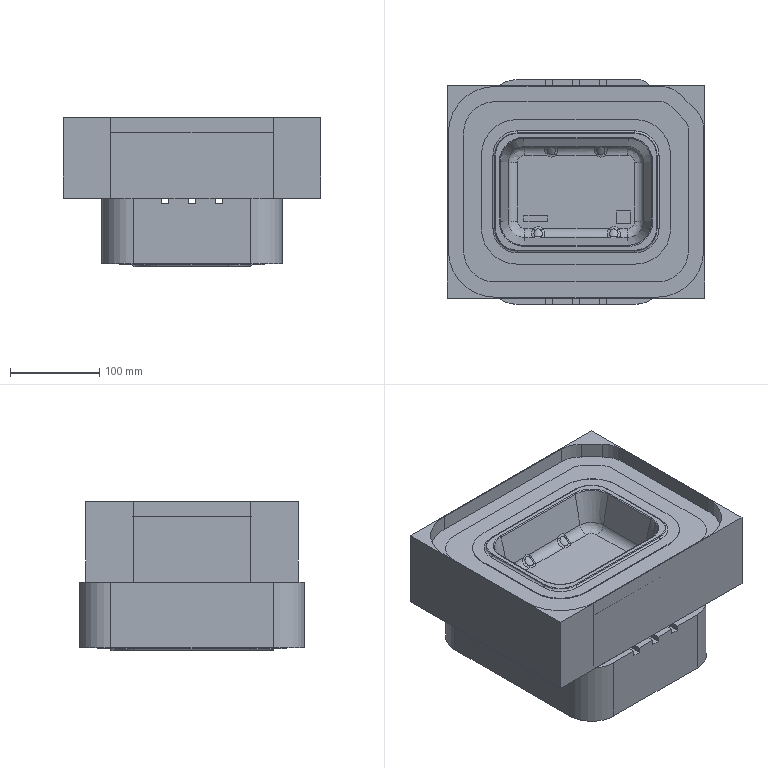NC program | NX | posted with a generic post | part box 287.436 x 251.436 x 167.016 mm
Lines 1 to 1276 of 118587:
N10 G17 G21 G94 G90
(01 , TOOL : D16R0.8)
N12 T00 M6
N14 G53
N16 G17 G0 G90 X27.566 Y-109.658 S7000 M3 M8
N18 G43 Z240.5 H0
N20 Z91.5
N22 G94 G1 X0. Z90.055 F4500.
N24 X-90.718
N26 G2 X-134.583 Y-65.793 R43.865
N28 G1 Y65.793
N30 G2 X-90.718 Y109.658 R43.865
N32 G1 X94.505
N34 G2 X111.38 Y102.668 R23.865
N36 G1 X127.593 Y86.455
N38 G2 X134.583 Y69.58 R23.865
N40 G1 Y-65.793
N42 G2 X90.718 Y-109.658 R43.865
N44 G1 X0.
N46 Y-99.578
N48 X-90.718
N50 G2 X-124.503 Y-65.793 R33.785
N52 G1 Y65.793
N54 G2 X-90.718 Y99.578 R33.785
N56 G1 X94.505
N58 G2 X104.252 Y95.541 R13.785
N60 G1 X120.466 Y79.327
N62 G2 X124.503 Y69.58 R13.785
N64 G1 Y-65.793
N66 G2 X90.718 Y-99.578 R33.785
N68 G1 X0.
N70 Y-89.498
N72 X-90.718
N74 G2 X-114.423 Y-65.793 R23.705
N76 G1 Y65.793
N78 G2 X-90.718 Y89.498 R23.705
N80 G1 X94.505
N82 G2 X97.125 Y88.413 R3.705
N84 G1 X113.338 Y72.2
N86 G2 X114.423 Y69.58 R3.705
N88 G1 Y-65.793
N90 G2 X90.718 Y-89.498 R23.705
N92 G1 X0.
N94 Y-79.418
N96 X-90.718
N98 G2 X-104.343 Y-65.793 R13.625
N100 G1 Y65.793
N102 G2 X-90.718 Y79.418 R13.625
N104 G1 X91.864
N106 X104.343 Y66.939
N108 Y-65.793
N110 G2 X90.718 Y-79.418 R13.625
N112 G1 X0.
N114 Y-69.338
N116 X-90.718
N118 G2 X-94.263 Y-65.793 R3.545
N120 G1 Y65.793
N122 G2 X-90.718 Y69.338 R3.545
N124 G1 X87.689
N126 X94.263 Y62.764
N128 Y-65.793
N130 G2 X90.718 Y-69.338 R3.545
N132 G1 X0.
N134 Y-59.258
N136 X-84.183
N138 Y59.258
N140 X83.514
N142 X84.183 Y58.589
N144 Y-59.258
N146 X0.
N148 Y-49.178
N150 X-74.103
N152 Y49.178
N154 X74.103
N156 Y-49.178
N158 X0.
N160 Y-39.098
N162 X-64.023
N164 Y39.098
N166 X64.023
N168 Y-39.098
N170 X0.
N172 Y-29.018
N174 X-53.943
N176 Y29.018
N178 X53.943
N180 Y-29.018
N182 X0.
N184 Y-18.938
N186 X-43.863
N188 Y18.938
N190 X43.863
N192 Y-18.938
N194 X0.
N196 Y-8.858
N198 X-33.783
N200 Y8.858
N202 X33.783
N204 Y-8.858
N206 X0.
N208 Y-1.658
N210 X-26.583
N212 Y1.658
N214 X26.583
N216 Y-1.658
N218 X0.
N220 G3 X-3.2 Y-4.858 R3.2
N222 G1 Z91.055
N224 G0 Z93.5
N226 X27.566 Y-109.593
N228 Z91.055
N230 G1 X0. Z89.611
N232 X-90.718
N234 G2 X-134.518 Y-65.793 R43.8
N236 G1 Y65.793
N238 G2 X-90.718 Y109.593 R43.8
N240 G1 X94.505
N242 G2 X111.334 Y102.622 R23.8
N244 G1 X127.547 Y86.409
N246 G2 X134.518 Y69.58 R23.8
N248 G1 Y-65.793
N250 G2 X90.718 Y-109.593 R43.8
N252 G1 X0.
N254 Y-99.513
N256 X-90.718
N258 G2 X-124.438 Y-65.793 R33.72
N260 G1 Y65.793
N262 G2 X-90.718 Y99.513 R33.72
N264 G1 X94.505
N266 G2 X104.206 Y95.495 R13.72
N268 G1 X120.42 Y79.281
N270 G2 X124.438 Y69.58 R13.72
N272 G1 Y-65.793
N274 G2 X90.718 Y-99.513 R33.72
N276 G1 X0.
N278 Y-89.433
N280 X-90.718
N282 G2 X-114.358 Y-65.793 R23.64
N284 G1 Y65.793
N286 G2 X-90.718 Y89.433 R23.64
N288 G1 X94.505
N290 G2 X97.079 Y88.367 R3.64
N292 G1 X113.292 Y72.154
N294 G2 X114.358 Y69.58 R3.64
N296 G1 Y-65.793
N298 G2 X90.718 Y-89.433 R23.64
N300 G1 X0.
N302 Y-79.353
N304 X-90.718
N306 G2 X-104.278 Y-65.793 R13.56
N308 G1 Y65.793
N310 G2 X-90.718 Y79.353 R13.56
N312 G1 X91.837
N314 X104.278 Y66.912
N316 Y-65.793
N318 G2 X90.718 Y-79.353 R13.56
N320 G1 X0.
N322 Y-69.273
N324 X-90.718
N326 G2 X-94.198 Y-65.793 R3.48
N328 G1 Y65.793
N330 G2 X-90.718 Y69.273 R3.48
N332 G1 X87.662
N334 X94.198 Y62.737
N336 Y-65.793
N338 G2 X90.718 Y-69.273 R3.48
N340 G1 X0.
N342 Y-59.193
N344 X-84.118
N346 Y59.193
N348 X83.487
N350 X84.118 Y58.562
N352 Y-59.193
N354 X0.
N356 Y-49.113
N358 X-74.038
N360 Y49.113
N362 X74.038
N364 Y-49.113
N366 X0.
N368 Y-39.033
N370 X-63.958
N372 Y39.033
N374 X63.958
N376 Y-39.033
N378 X0.
N380 Y-28.953
N382 X-53.878
N384 Y28.953
N386 X53.878
N388 Y-28.953
N390 X0.
N392 Y-18.873
N394 X-43.798
N396 Y18.873
N398 X43.798
N400 Y-18.873
N402 X0.
N404 Y-8.793
N406 X-33.718
N408 Y8.793
N410 X33.718
N412 Y-8.793
N414 X0.
N416 Y-1.593
N418 X-26.518
N420 Y1.593
N422 X26.518
N424 Y-1.593
N426 X0.
N428 G3 X-3.2 Y-4.793 R3.2
N430 G1 Z90.611
N432 G0 Z93.055
N434 X27.566 Y-109.593
N436 Z90.611
N438 G1 X0. Z89.166
N440 X-90.718
N442 G2 X-134.518 Y-65.793 R43.8
N444 G1 Y65.793
N446 G2 X-90.718 Y109.593 R43.8
N448 G1 X94.505
N450 G2 X111.334 Y102.622 R23.8
N452 G1 X127.547 Y86.409
N454 G2 X134.518 Y69.58 R23.8
N456 G1 Y-65.793
N458 G2 X90.718 Y-109.593 R43.8
N460 G1 X0.
N462 Y-99.513
N464 X-90.718
N466 G2 X-124.438 Y-65.793 R33.72
N468 G1 Y65.793
N470 G2 X-90.718 Y99.513 R33.72
N472 G1 X94.505
N474 G2 X104.206 Y95.495 R13.72
N476 G1 X120.42 Y79.281
N478 G2 X124.438 Y69.58 R13.72
N480 G1 Y-65.793
N482 G2 X90.718 Y-99.513 R33.72
N484 G1 X0.
N486 Y-89.433
N488 X-90.718
N490 G2 X-114.358 Y-65.793 R23.64
N492 G1 Y65.793
N494 G2 X-90.718 Y89.433 R23.64
N496 G1 X94.505
N498 G2 X97.079 Y88.367 R3.64
N500 G1 X113.292 Y72.154
N502 G2 X114.358 Y69.58 R3.64
N504 G1 Y-65.793
N506 G2 X90.718 Y-89.433 R23.64
N508 G1 X0.
N510 Y-79.353
N512 X-90.718
N514 G2 X-104.278 Y-65.793 R13.56
N516 G1 Y65.793
N518 G2 X-90.718 Y79.353 R13.56
N520 G1 X91.837
N522 X104.278 Y66.912
N524 Y-65.793
N526 G2 X90.718 Y-79.353 R13.56
N528 G1 X0.
N530 Y-69.273
N532 X-90.718
N534 G2 X-94.198 Y-65.793 R3.48
N536 G1 Y65.793
N538 G2 X-90.718 Y69.273 R3.48
N540 G1 X87.662
N542 X94.198 Y62.737
N544 Y-65.793
N546 G2 X90.718 Y-69.273 R3.48
N548 G1 X0.
N550 Y-59.193
N552 X-84.118
N554 Y59.193
N556 X83.487
N558 X84.118 Y58.562
N560 Y-59.193
N562 X0.
N564 Y-49.113
N566 X-74.038
N568 Y49.113
N570 X74.038
N572 Y-49.113
N574 X0.
N576 Y-39.033
N578 X-63.958
N580 Y39.033
N582 X63.958
N584 Y-39.033
N586 X0.
N588 Y-28.953
N590 X-53.878
N592 Y28.953
N594 X53.878
N596 Y-28.953
N598 X0.
N600 Y-18.873
N602 X-43.798
N604 Y18.873
N606 X43.798
N608 Y-18.873
N610 X0.
N612 Y-8.793
N614 X-33.718
N616 Y8.793
N618 X33.718
N620 Y-8.793
N622 X0.
N624 Y-1.593
N626 X-26.518
N628 Y1.593
N630 X26.518
N632 Y-1.593
N634 X0.
N636 G3 X-3.2 Y-4.793 R3.2
N638 G1 Z90.166
N640 G0 Z92.611
N642 X27.566 Y-109.593
N644 Z90.166
N646 G1 X0. Z88.721
N648 X-90.718
N650 G2 X-134.518 Y-65.793 R43.8
N652 G1 Y65.793
N654 G2 X-90.718 Y109.593 R43.8
N656 G1 X94.505
N658 G2 X111.334 Y102.622 R23.8
N660 G1 X127.547 Y86.409
N662 G2 X134.518 Y69.58 R23.8
N664 G1 Y-65.793
N666 G2 X90.718 Y-109.593 R43.8
N668 G1 X0.
N670 Y-99.513
N672 X-90.718
N674 G2 X-124.438 Y-65.793 R33.72
N676 G1 Y65.793
N678 G2 X-90.718 Y99.513 R33.72
N680 G1 X94.505
N682 G2 X104.206 Y95.495 R13.72
N684 G1 X120.42 Y79.281
N686 G2 X124.438 Y69.58 R13.72
N688 G1 Y-65.793
N690 G2 X90.718 Y-99.513 R33.72
N692 G1 X0.
N694 Y-89.433
N696 X-90.718
N698 G2 X-114.358 Y-65.793 R23.64
N700 G1 Y65.793
N702 G2 X-90.718 Y89.433 R23.64
N704 G1 X94.505
N706 G2 X97.079 Y88.367 R3.64
N708 G1 X113.292 Y72.154
N710 G2 X114.358 Y69.58 R3.64
N712 G1 Y-65.793
N714 G2 X90.718 Y-89.433 R23.64
N716 G1 X0.
N718 Y-79.353
N720 X-90.718
N722 G2 X-104.278 Y-65.793 R13.56
N724 G1 Y65.793
N726 G2 X-90.718 Y79.353 R13.56
N728 G1 X91.837
N730 X104.278 Y66.912
N732 Y-65.793
N734 G2 X90.718 Y-79.353 R13.56
N736 G1 X0.
N738 Y-69.273
N740 X-90.718
N742 G2 X-94.198 Y-65.793 R3.48
N744 G1 Y65.793
N746 G2 X-90.718 Y69.273 R3.48
N748 G1 X87.662
N750 X94.198 Y62.737
N752 Y-65.793
N754 G2 X90.718 Y-69.273 R3.48
N756 G1 X0.
N758 Y-59.193
N760 X-84.118
N762 Y59.193
N764 X83.487
N766 X84.118 Y58.562
N768 Y-59.193
N770 X0.
N772 Y-49.113
N774 X-74.038
N776 Y49.113
N778 X74.038
N780 Y-49.113
N782 X0.
N784 Y-39.033
N786 X-63.958
N788 Y39.033
N790 X63.958
N792 Y-39.033
N794 X0.
N796 Y-28.953
N798 X-53.878
N800 Y28.953
N802 X53.878
N804 Y-28.953
N806 X0.
N808 Y-18.873
N810 X-43.798
N812 Y18.873
N814 X43.798
N816 Y-18.873
N818 X0.
N820 Y-8.793
N822 X-33.718
N824 Y8.793
N826 X33.718
N828 Y-8.793
N830 X0.
N832 Y-1.593
N834 X-26.518
N836 Y1.593
N838 X26.518
N840 Y-1.593
N842 X0.
N844 G3 X-3.2 Y-4.793 R3.2
N846 G1 Z89.721
N848 G0 Z92.166
N850 X27.566 Y-109.593
N852 Z89.721
N854 G1 X0. Z88.277
N856 X-90.718
N858 G2 X-134.518 Y-65.793 R43.8
N860 G1 Y65.793
N862 G2 X-90.718 Y109.593 R43.8
N864 G1 X94.505
N866 G2 X111.334 Y102.622 R23.8
N868 G1 X127.547 Y86.409
N870 G2 X134.518 Y69.58 R23.8
N872 G1 Y-65.793
N874 G2 X90.718 Y-109.593 R43.8
N876 G1 X0.
N878 Y-99.513
N880 X-90.718
N882 G2 X-124.438 Y-65.793 R33.72
N884 G1 Y65.793
N886 G2 X-90.718 Y99.513 R33.72
N888 G1 X94.505
N890 G2 X104.206 Y95.495 R13.72
N892 G1 X120.42 Y79.281
N894 G2 X124.438 Y69.58 R13.72
N896 G1 Y-65.793
N898 G2 X90.718 Y-99.513 R33.72
N900 G1 X0.
N902 Y-89.433
N904 X-90.718
N906 G2 X-114.358 Y-65.793 R23.64
N908 G1 Y65.793
N910 G2 X-90.718 Y89.433 R23.64
N912 G1 X94.505
N914 G2 X97.079 Y88.367 R3.64
N916 G1 X113.292 Y72.154
N918 G2 X114.358 Y69.58 R3.64
N920 G1 Y-65.793
N922 G2 X90.718 Y-89.433 R23.64
N924 G1 X0.
N926 Y-79.353
N928 X-90.718
N930 G2 X-104.278 Y-65.793 R13.56
N932 G1 Y65.793
N934 G2 X-90.718 Y79.353 R13.56
N936 G1 X91.837
N938 X104.278 Y66.912
N940 Y-65.793
N942 G2 X90.718 Y-79.353 R13.56
N944 G1 X0.
N946 Y-69.273
N948 X-90.718
N950 G2 X-94.198 Y-65.793 R3.48
N952 G1 Y65.793
N954 G2 X-90.718 Y69.273 R3.48
N956 G1 X87.662
N958 X94.198 Y62.737
N960 Y-65.793
N962 G2 X90.718 Y-69.273 R3.48
N964 G1 X0.
N966 Y-59.193
N968 X-84.118
N970 Y59.193
N972 X83.487
N974 X84.118 Y58.562
N976 Y-59.193
N978 X0.
N980 Y-49.113
N982 X-74.038
N984 Y49.113
N986 X74.038
N988 Y-49.113
N990 X0.
N992 Y-39.033
N994 X-63.958
N996 Y39.033
N998 X63.958
N1000 Y-39.033
N1002 X0.
N1004 Y-28.953
N1006 X-53.878
N1008 Y28.953
N1010 X53.878
N1012 Y-28.953
N1014 X0.
N1016 Y-18.873
N1018 X-43.798
N1020 Y18.873
N1022 X43.798
N1024 Y-18.873
N1026 X0.
N1028 Y-8.793
N1030 X-33.718
N1032 Y8.793
N1034 X33.718
N1036 Y-8.793
N1038 X0.
N1040 Y-1.593
N1042 X-26.518
N1044 Y1.593
N1046 X26.518
N1048 Y-1.593
N1050 X0.
N1052 G3 X-3.2 Y-4.793 R3.2
N1054 G1 Z89.277
N1056 G0 Z91.721
N1058 X27.566 Y-109.593
N1060 Z89.277
N1062 G1 X0. Z87.832
N1064 X-90.718
N1066 G2 X-134.518 Y-65.793 R43.8
N1068 G1 Y65.793
N1070 G2 X-90.718 Y109.593 R43.8
N1072 G1 X94.505
N1074 G2 X111.334 Y102.622 R23.8
N1076 G1 X127.547 Y86.409
N1078 G2 X134.518 Y69.58 R23.8
N1080 G1 Y-65.793
N1082 G2 X90.718 Y-109.593 R43.8
N1084 G1 X0.
N1086 Y-99.513
N1088 X-90.718
N1090 G2 X-124.438 Y-65.793 R33.72
N1092 G1 Y65.793
N1094 G2 X-90.718 Y99.513 R33.72
N1096 G1 X94.505
N1098 G2 X104.206 Y95.495 R13.72
N1100 G1 X120.42 Y79.281
N1102 G2 X124.438 Y69.58 R13.72
N1104 G1 Y-65.793
N1106 G2 X90.718 Y-99.513 R33.72
N1108 G1 X0.
N1110 Y-89.433
N1112 X-90.718
N1114 G2 X-114.358 Y-65.793 R23.64
N1116 G1 Y65.793
N1118 G2 X-90.718 Y89.433 R23.64
N1120 G1 X94.505
N1122 G2 X97.079 Y88.367 R3.64
N1124 G1 X113.292 Y72.154
N1126 G2 X114.358 Y69.58 R3.64
N1128 G1 Y-65.793
N1130 G2 X90.718 Y-89.433 R23.64
N1132 G1 X0.
N1134 Y-79.353
N1136 X-90.718
N1138 G2 X-104.278 Y-65.793 R13.56
N1140 G1 Y65.793
N1142 G2 X-90.718 Y79.353 R13.56
N1144 G1 X91.837
N1146 X104.278 Y66.912
N1148 Y-65.793
N1150 G2 X90.718 Y-79.353 R13.56
N1152 G1 X0.
N1154 Y-69.273
N1156 X-90.718
N1158 G2 X-94.198 Y-65.793 R3.48
N1160 G1 Y65.793
N1162 G2 X-90.718 Y69.273 R3.48
N1164 G1 X87.662
N1166 X94.198 Y62.737
N1168 Y-65.793
N1170 G2 X90.718 Y-69.273 R3.48
N1172 G1 X0.
N1174 Y-59.193
N1176 X-84.118
N1178 Y59.193
N1180 X83.487
N1182 X84.118 Y58.562
N1184 Y-59.193
N1186 X0.
N1188 Y-49.113
N1190 X-74.038
N1192 Y49.113
N1194 X74.038
N1196 Y-49.113
N1198 X0.
N1200 Y-39.033
N1202 X-63.958
N1204 Y39.033
N1206 X63.958
N1208 Y-39.033
N1210 X0.
N1212 Y-28.953
N1214 X-53.878
N1216 Y28.953
N1218 X53.878
N1220 Y-28.953
N1222 X0.
N1224 Y-18.873
N1226 X-43.798
N1228 Y18.873
N1230 X43.798
N1232 Y-18.873
N1234 X0.
N1236 Y-8.793
N1238 X-33.718
N1240 Y8.793
N1242 X33.718
N1244 Y-8.793
N1246 X0.
N1248 Y-1.593
N1250 X-26.518
N1252 Y1.593
N1254 X26.518
N1256 Y-1.593
N1258 X0.
N1260 G3 X-3.2 Y-4.793 R3.2
N1262 G1 Z88.832
N1264 G0 Z91.277
N1266 X27.566 Y-109.593
N1268 Z88.832
N1270 G1 X0. Z87.387
N1272 X-90.718
N1274 G2 X-134.518 Y-65.793 R43.8
N1276 G1 Y65.793
N1278 G2 X-90.718 Y109.593 R43.8
N1280 G1 X94.505
N1282 G2 X111.334 Y102.622 R23.8
N1284 G1 X127.547 Y86.409
N1286 G2 X134.518 Y69.58 R23.8
N1288 G1 Y-65.793
N1290 G2 X90.718 Y-109.593 R43.8
N1292 G1 X0.
N1294 Y-99.513
N1296 X-90.718
N1298 G2 X-124.438 Y-65.793 R33.72
N1300 G1 Y65.793
N1302 G2 X-90.718 Y99.513 R33.72
N1304 G1 X94.505
N1306 G2 X104.206 Y95.495 R13.72
N1308 G1 X120.42 Y79.281
N1310 G2 X124.438 Y69.58 R13.72
N1312 G1 Y-65.793
N1314 G2 X90.718 Y-99.513 R33.72
N1316 G1 X0.
N1318 Y-89.433
N1320 X-90.718
N1322 G2 X-114.358 Y-65.793 R23.64
N1324 G1 Y65.793
N1326 G2 X-90.718 Y89.433 R23.64
N1328 G1 X94.505
N1330 G2 X97.079 Y88.367 R3.64
N1332 G1 X113.292 Y72.154
N1334 G2 X114.358 Y69.58 R3.64
N1336 G1 Y-65.793
N1338 G2 X90.718 Y-89.433 R23.64
N1340 G1 X0.
N1342 Y-79.353
N1344 X-90.718
N1346 G2 X-104.278 Y-65.793 R13.56
N1348 G1 Y65.793
N1350 G2 X-90.718 Y79.353 R13.56
N1352 G1 X91.837
N1354 X104.278 Y66.912
N1356 Y-65.793
N1358 G2 X90.718 Y-79.353 R13.56
N1360 G1 X0.
N1362 Y-69.273
N1364 X-90.718
N1366 G2 X-94.198 Y-65.793 R3.48
N1368 G1 Y65.793
N1370 G2 X-90.718 Y69.273 R3.48
N1372 G1 X87.662
N1374 X94.198 Y62.737
N1376 Y-65.793
N1378 G2 X90.718 Y-69.273 R3.48
N1380 G1 X0.
N1382 Y-59.193
N1384 X-84.118
N1386 Y59.193
N1388 X83.487
N1390 X84.118 Y58.562
N1392 Y-59.193
N1394 X0.
N1396 Y-49.113
N1398 X-74.038
N1400 Y49.113
N1402 X74.038
N1404 Y-49.113
N1406 X0.
N1408 Y-39.033
N1410 X-63.958
N1412 Y39.033
N1414 X63.958
N1416 Y-39.033
N1418 X0.
N1420 Y-28.953
N1422 X-53.878
N1424 Y28.953
N1426 X53.878
N1428 Y-28.953
N1430 X0.
N1432 Y-18.873
N1434 X-43.798
N1436 Y18.873
N1438 X43.798
N1440 Y-18.873
N1442 X0.
N1444 Y-8.793
N1446 X-33.718
N1448 Y8.793
N1450 X33.718
N1452 Y-8.793
N1454 X0.
N1456 Y-1.593
N1458 X-26.518
N1460 Y1.593
N1462 X26.518
N1464 Y-1.593
N1466 X0.
N1468 G3 X-3.2 Y-4.793 R3.2
N1470 G1 Z88.387
N1472 G0 Z90.832
N1474 X27.566 Y-109.593
N1476 Z88.387
N1478 G1 X0. Z86.943
N1480 X-90.718
N1482 G2 X-134.518 Y-65.793 R43.8
N1484 G1 Y65.793
N1486 G2 X-90.718 Y109.593 R43.8
N1488 G1 X94.505
N1490 G2 X111.334 Y102.622 R23.8
N1492 G1 X127.547 Y86.409
N1494 G2 X134.518 Y69.58 R23.8
N1496 G1 Y-65.793
N1498 G2 X90.718 Y-109.593 R43.8
N1500 G1 X0.
N1502 Y-99.513
N1504 X-90.718
N1506 G2 X-124.438 Y-65.793 R33.72
N1508 G1 Y65.793
N1510 G2 X-90.718 Y99.513 R33.72
N1512 G1 X94.505
N1514 G2 X104.206 Y95.495 R13.72
N1516 G1 X120.42 Y79.281
N1518 G2 X124.438 Y69.58 R13.72
N1520 G1 Y-65.793
N1522 G2 X90.718 Y-99.513 R33.72
N1524 G1 X0.
N1526 Y-89.433
N1528 X-90.718
N1530 G2 X-114.358 Y-65.793 R23.64
N1532 G1 Y65.793
N1534 G2 X-90.718 Y89.433 R23.64
N1536 G1 X94.505
N1538 G2 X97.079 Y88.367 R3.64
N1540 G1 X113.292 Y72.154
N1542 G2 X114.358 Y69.58 R3.64
N1544 G1 Y-65.793
N1546 G2 X90.718 Y-89.433 R23.64
N1548 G1 X0.
N1550 Y-79.353
N1552 X-90.718
N1554 G2 X-104.278 Y-65.793 R13.56
N1556 G1 Y65.793
N1558 G2 X-90.718 Y79.353 R13.56
N1560 G1 X91.837
N1562 X104.278 Y66.912
N1564 Y-65.793
N1566 G2 X90.718 Y-79.353 R13.56
N1568 G1 X0.
N1570 Y-69.273
N1572 X-90.718
N1574 G2 X-94.198 Y-65.793 R3.48
N1576 G1 Y65.793
N1578 G2 X-90.718 Y69.273 R3.48
N1580 G1 X87.662
N1582 X94.198 Y62.737
N1584 Y-65.793
N1586 G2 X90.718 Y-69.273 R3.48
N1588 G1 X0.
N1590 Y-59.193
N1592 X-84.118
N1594 Y59.193
N1596 X83.487
N1598 X84.118 Y58.562
N1600 Y-59.193
N1602 X0.
N1604 Y-49.113
N1606 X-74.038
N1608 Y49.113
N1610 X74.038
N1612 Y-49.113
N1614 X0.
N1616 Y-39.033
N1618 X-63.958
N1620 Y39.033
N1622 X63.958
N1624 Y-39.033
N1626 X0.
N1628 Y-28.953
N1630 X-53.878
N1632 Y28.953
N1634 X53.878
N1636 Y-28.953
N1638 X0.
N1640 Y-18.873
N1642 X-43.798
N1644 Y18.873
N1646 X43.798
N1648 Y-18.873
N1650 X0.
N1652 Y-8.793
N1654 X-33.718
N1656 Y8.793
N1658 X33.718
N1660 Y-8.793
N1662 X0.
N1664 Y-1.593
N1666 X-26.518
N1668 Y1.593
N1670 X26.518
N1672 Y-1.593
N1674 X0.
N1676 G3 X-3.2 Y-4.793 R3.2
N1678 G1 Z87.943
N1680 G0 Z90.387
N1682 X27.566 Y-109.593
N1684 Z87.943
N1686 G1 X0. Z86.498
N1688 X-90.718
N1690 G2 X-134.518 Y-65.793 R43.8
N1692 G1 Y65.793
N1694 G2 X-90.718 Y109.593 R43.8
N1696 G1 X94.505
N1698 G2 X111.334 Y102.622 R23.8
N1700 G1 X127.547 Y86.409
N1702 G2 X134.518 Y69.58 R23.8
N1704 G1 Y-65.793
N1706 G2 X90.718 Y-109.593 R43.8
N1708 G1 X0.
N1710 Y-99.513
N1712 X-90.718
N1714 G2 X-124.438 Y-65.793 R33.72
N1716 G1 Y65.793
N1718 G2 X-90.718 Y99.513 R33.72
N1720 G1 X94.505
N1722 G2 X104.206 Y95.495 R13.72
N1724 G1 X120.42 Y79.281
N1726 G2 X124.438 Y69.58 R13.72
N1728 G1 Y-65.793
N1730 G2 X90.718 Y-99.513 R33.72
N1732 G1 X0.
N1734 Y-89.433
N1736 X-90.718
N1738 G2 X-114.358 Y-65.793 R23.64
N1740 G1 Y65.793
N1742 G2 X-90.718 Y89.433 R23.64
N1744 G1 X94.505
N1746 G2 X97.079 Y88.367 R3.64
N1748 G1 X113.292 Y72.154
N1750 G2 X114.358 Y69.58 R3.64
N1752 G1 Y-65.793
N1754 G2 X90.718 Y-89.433 R23.64
N1756 G1 X0.
N1758 Y-79.353
N1760 X-90.718
N1762 G2 X-104.278 Y-65.793 R13.56
N1764 G1 Y65.793
N1766 G2 X-90.718 Y79.353 R13.56
N1768 G1 X91.837
N1770 X104.278 Y66.912
N1772 Y-65.793
N1774 G2 X90.718 Y-79.353 R13.56
N1776 G1 X0.
N1778 Y-69.273
N1780 X-90.718
N1782 G2 X-94.198 Y-65.793 R3.48
N1784 G1 Y65.793
N1786 G2 X-90.718 Y69.273 R3.48
N1788 G1 X87.662
N1790 X94.198 Y62.737
N1792 Y-65.793
N1794 G2 X90.718 Y-69.273 R3.48
N1796 G1 X0.
N1798 Y-59.193
N1800 X-84.118
N1802 Y59.193
N1804 X83.487
N1806 X84.118 Y58.562
N1808 Y-59.193
N1810 X0.
N1812 Y-49.113
N1814 X-74.038
N1816 Y49.113
N1818 X74.038
N1820 Y-49.113
N1822 X0.
N1824 Y-39.033
N1826 X-63.958
N1828 Y39.033
N1830 X63.958
N1832 Y-39.033
N1834 X0.
N1836 Y-28.953
N1838 X-53.878
N1840 Y28.953
N1842 X53.878
N1844 Y-28.953
N1846 X0.
N1848 Y-18.873
N1850 X-43.798
N1852 Y18.873
N1854 X43.798
N1856 Y-18.873
N1858 X0.
N1860 Y-8.793
N1862 X-33.718
N1864 Y8.793
N1866 X33.718
N1868 Y-8.793
N1870 X0.
N1872 Y-1.593
N1874 X-26.518
N1876 Y1.593
N1878 X26.518
N1880 Y-1.593
N1882 X0.
N1884 G3 X-3.2 Y-4.793 R3.2
N1886 G1 Z87.498
N1888 G0 Z89.943
N1890 X27.566 Y-109.593
N1892 Z87.498
N1894 G1 X0. Z86.053
N1896 X-90.718
N1898 G2 X-134.518 Y-65.793 R43.8
N1900 G1 Y65.793
N1902 G2 X-90.718 Y109.593 R43.8
N1904 G1 X94.505
N1906 G2 X111.334 Y102.622 R23.8
N1908 G1 X127.547 Y86.409
N1910 G2 X134.518 Y69.58 R23.8
N1912 G1 Y-65.793
N1914 G2 X90.718 Y-109.593 R43.8
N1916 G1 X0.
N1918 Y-99.513
N1920 X-90.718
N1922 G2 X-124.438 Y-65.793 R33.72
N1924 G1 Y65.793
N1926 G2 X-90.718 Y99.513 R33.72
N1928 G1 X94.505
N1930 G2 X104.206 Y95.495 R13.72
N1932 G1 X120.42 Y79.281
N1934 G2 X124.438 Y69.58 R13.72
N1936 G1 Y-65.793
N1938 G2 X90.718 Y-99.513 R33.72
N1940 G1 X0.
N1942 Y-89.433
N1944 X-90.718
N1946 G2 X-114.358 Y-65.793 R23.64
N1948 G1 Y65.793
N1950 G2 X-90.718 Y89.433 R23.64
N1952 G1 X94.505
N1954 G2 X97.079 Y88.367 R3.64
N1956 G1 X113.292 Y72.154
N1958 G2 X114.358 Y69.58 R3.64
N1960 G1 Y-65.793
N1962 G2 X90.718 Y-89.433 R23.64
N1964 G1 X0.
N1966 Y-79.353
N1968 X-90.718
N1970 G2 X-104.278 Y-65.793 R13.56
N1972 G1 Y65.793
N1974 G2 X-90.718 Y79.353 R13.56
N1976 G1 X91.837
N1978 X104.278 Y66.912
N1980 Y-65.793
N1982 G2 X90.718 Y-79.353 R13.56
N1984 G1 X0.
N1986 Y-69.273
N1988 X-90.718
N1990 G2 X-94.198 Y-65.793 R3.48
N1992 G1 Y65.793
N1994 G2 X-90.718 Y69.273 R3.48
N1996 G1 X87.662
N1998 X94.198 Y62.737
N2000 Y-65.793
N2002 G2 X90.718 Y-69.273 R3.48
N2004 G1 X0.
N2006 Y-59.193
N2008 X-84.118
N2010 Y59.193
N2012 X83.487
N2014 X84.118 Y58.562
N2016 Y-59.193
N2018 X0.
N2020 Y-49.113
N2022 X-74.038
N2024 Y49.113
N2026 X74.038
N2028 Y-49.113
N2030 X0.
N2032 Y-39.033
N2034 X-63.958
N2036 Y39.033
N2038 X63.958
N2040 Y-39.033
N2042 X0.
N2044 Y-28.953
N2046 X-53.878
N2048 Y28.953
N2050 X53.878
N2052 Y-28.953
N2054 X0.
N2056 Y-18.873
N2058 X-43.798
N2060 Y18.873
N2062 X43.798
N2064 Y-18.873
N2066 X0.
N2068 Y-8.793
N2070 X-33.718
N2072 Y8.793
N2074 X33.718
N2076 Y-8.793
N2078 X0.
N2080 Y-1.593
N2082 X-26.518
N2084 Y1.593
N2086 X26.518
N2088 Y-1.593
N2090 X0.
N2092 G3 X-3.2 Y-4.793 R3.2
N2094 G1 Z87.053
N2096 G0 Z89.498
N2098 X27.566 Y-109.593
N2100 Z87.053
N2102 G1 X0. Z85.609
N2104 X-90.718
N2106 G2 X-134.518 Y-65.793 R43.8
N2108 G1 Y65.793
N2110 G2 X-90.718 Y109.593 R43.8
N2112 G1 X94.505
N2114 G2 X111.334 Y102.622 R23.8
N2116 G1 X127.547 Y86.409
N2118 G2 X134.518 Y69.58 R23.8
N2120 G1 Y-65.793
N2122 G2 X90.718 Y-109.593 R43.8
N2124 G1 X0.
N2126 Y-99.513
N2128 X-90.718
N2130 G2 X-124.438 Y-65.793 R33.72
N2132 G1 Y65.793
N2134 G2 X-90.718 Y99.513 R33.72
N2136 G1 X94.505
N2138 G2 X104.206 Y95.495 R13.72
N2140 G1 X120.42 Y79.281
N2142 G2 X124.438 Y69.58 R13.72
N2144 G1 Y-65.793
N2146 G2 X90.718 Y-99.513 R33.72
N2148 G1 X0.
N2150 Y-89.433
N2152 X-90.718
N2154 G2 X-114.358 Y-65.793 R23.64
N2156 G1 Y65.793
N2158 G2 X-90.718 Y89.433 R23.64
N2160 G1 X94.505
N2162 G2 X97.079 Y88.367 R3.64
N2164 G1 X113.292 Y72.154
N2166 G2 X114.358 Y69.58 R3.64
N2168 G1 Y-65.793
N2170 G2 X90.718 Y-89.433 R23.64
N2172 G1 X0.
N2174 Y-79.353
N2176 X-90.718
N2178 G2 X-104.278 Y-65.793 R13.56
N2180 G1 Y65.793
N2182 G2 X-90.718 Y79.353 R13.56
N2184 G1 X91.837
N2186 X104.278 Y66.912
N2188 Y-65.793
N2190 G2 X90.718 Y-79.353 R13.56
N2192 G1 X0.
N2194 Y-69.273
N2196 X-90.718
N2198 G2 X-94.198 Y-65.793 R3.48
N2200 G1 Y65.793
N2202 G2 X-90.718 Y69.273 R3.48
N2204 G1 X87.662
N2206 X94.198 Y62.737
N2208 Y-65.793
N2210 G2 X90.718 Y-69.273 R3.48
N2212 G1 X0.
N2214 Y-59.193
N2216 X-84.118
N2218 Y59.193
N2220 X83.487
N2222 X84.118 Y58.562
N2224 Y-59.193
N2226 X0.
N2228 Y-49.113
N2230 X-74.038
N2232 Y49.113
N2234 X74.038
N2236 Y-49.113
N2238 X0.
N2240 Y-39.033
N2242 X-63.958
N2244 Y39.033
N2246 X63.958
N2248 Y-39.033
N2250 X0.
N2252 Y-28.953
N2254 X-53.878
N2256 Y28.953
N2258 X53.878
N2260 Y-28.953
N2262 X0.
N2264 Y-18.873
N2266 X-43.798
N2268 Y18.873
N2270 X43.798
N2272 Y-18.873
N2274 X0.
N2276 Y-8.793
N2278 X-33.718
N2280 Y8.793
N2282 X33.718
N2284 Y-8.793
N2286 X0.
N2288 Y-1.593
N2290 X-26.518
N2292 Y1.593
N2294 X26.518
N2296 Y-1.593
N2298 X0.
N2300 G3 X-3.2 Y-4.793 R3.2
N2302 G1 Z86.609
N2304 G0 Z89.053
N2306 X27.566 Y-109.593
N2308 Z86.609
N2310 G1 X0. Z85.164
N2312 X-90.718
N2314 G2 X-134.518 Y-65.793 R43.8
N2316 G1 Y65.793
N2318 G2 X-90.718 Y109.593 R43.8
N2320 G1 X94.505
N2322 G2 X111.334 Y102.622 R23.8
N2324 G1 X127.547 Y86.409
N2326 G2 X134.518 Y69.58 R23.8
N2328 G1 Y-65.793
N2330 G2 X90.718 Y-109.593 R43.8
N2332 G1 X0.
N2334 Y-99.513
N2336 X-90.718
N2338 G2 X-124.438 Y-65.793 R33.72
N2340 G1 Y65.793
N2342 G2 X-90.718 Y99.513 R33.72
N2344 G1 X94.505
N2346 G2 X104.206 Y95.495 R13.72
N2348 G1 X120.42 Y79.281
N2350 G2 X124.438 Y69.58 R13.72
N2352 G1 Y-65.793
N2354 G2 X90.718 Y-99.513 R33.72
N2356 G1 X0.
N2358 Y-89.433
N2360 X-90.718
N2362 G2 X-114.358 Y-65.793 R23.64
N2364 G1 Y65.793
N2366 G2 X-90.718 Y89.433 R23.64
N2368 G1 X94.505
N2370 G2 X97.079 Y88.367 R3.64
N2372 G1 X113.292 Y72.154
N2374 G2 X114.358 Y69.58 R3.64
N2376 G1 Y-65.793
N2378 G2 X90.718 Y-89.433 R23.64
N2380 G1 X0.
N2382 Y-79.353
N2384 X-90.718
N2386 G2 X-104.278 Y-65.793 R13.56
N2388 G1 Y65.793
N2390 G2 X-90.718 Y79.353 R13.56
N2392 G1 X91.837
N2394 X104.278 Y66.912
N2396 Y-65.793
N2398 G2 X90.718 Y-79.353 R13.56
N2400 G1 X0.
N2402 Y-69.273
N2404 X-90.718
N2406 G2 X-94.198 Y-65.793 R3.48
N2408 G1 Y65.793
N2410 G2 X-90.718 Y69.273 R3.48
N2412 G1 X87.662
N2414 X94.198 Y62.737
N2416 Y-65.793
N2418 G2 X90.718 Y-69.273 R3.48
N2420 G1 X0.
N2422 Y-59.193
N2424 X-84.118
N2426 Y59.193
N2428 X83.487
N2430 X84.118 Y58.562
N2432 Y-59.193
N2434 X0.
N2436 Y-49.113
N2438 X-74.038
N2440 Y49.113
N2442 X74.038
N2444 Y-49.113
N2446 X0.
N2448 Y-39.033
N2450 X-63.958
N2452 Y39.033
N2454 X63.958
N2456 Y-39.033
N2458 X0.
N2460 Y-28.953
N2462 X-53.878
N2464 Y28.953
N2466 X53.878
N2468 Y-28.953
N2470 X0.
N2472 Y-18.873
N2474 X-43.798
N2476 Y18.873
N2478 X43.798
N2480 Y-18.873
N2482 X0.
N2484 Y-8.793
N2486 X-33.718
N2488 Y8.793
N2490 X33.718
N2492 Y-8.793
N2494 X0.
N2496 Y-1.593
N2498 X-26.518
N2500 Y1.593
N2502 X26.518
N2504 Y-1.593
N2506 X0.
N2508 G3 X-3.2 Y-4.793 R3.2
N2510 G1 Z86.164
N2512 G0 Z88.609
N2514 X27.566 Y-109.593
N2516 Z86.164
N2518 G1 X0. Z84.72
N2520 X-90.718
N2522 G2 X-134.518 Y-65.793 R43.8
N2524 G1 Y65.793
N2526 G2 X-90.718 Y109.593 R43.8
N2528 G1 X94.505
N2530 G2 X111.334 Y102.622 R23.8
N2532 G1 X127.547 Y86.409
N2534 G2 X134.518 Y69.58 R23.8
N2536 G1 Y-65.793
N2538 G2 X90.718 Y-109.593 R43.8
N2540 G1 X0.
N2542 Y-99.513
N2544 X-90.718
N2546 G2 X-124.438 Y-65.793 R33.72
N2548 G1 Y65.793
N2550 G2 X-90.718 Y99.513 R33.72